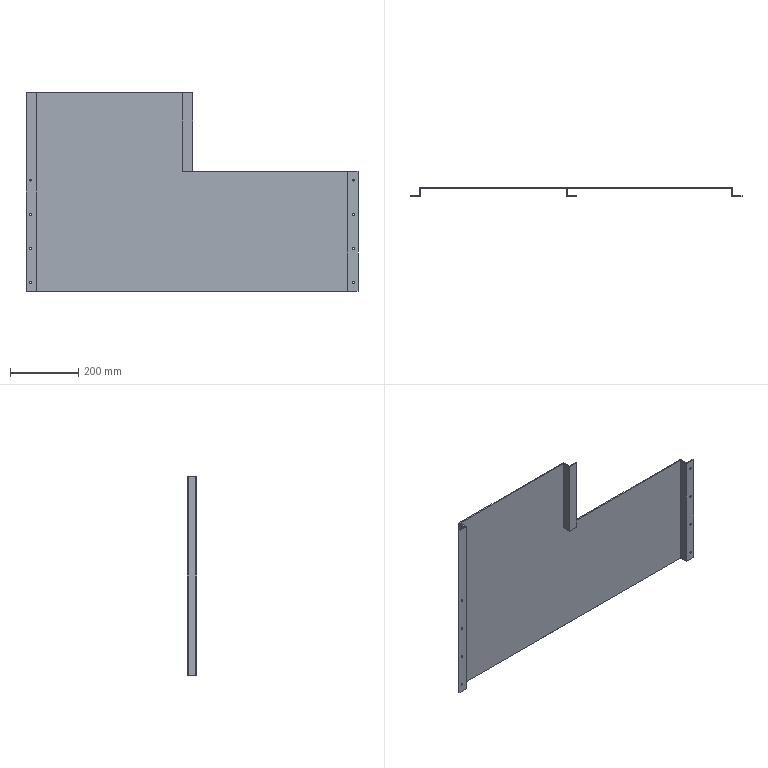Part | STEP file | Cutting guard | 1 solid | 37 faces | box 970 x 28 x 580 mm | volume 1440851 mm3 | plane 21 | cylinder 16 | commonest cylinder face diameters 6 x16
STEP:
#1=CARTESIAN_POINT('',(469.,-25.,-50.));
#2=VERTEX_POINT('',#1);
#3=CARTESIAN_POINT('',(475.,-25.,-50.));
#4=VERTEX_POINT('',#3);
#5=CARTESIAN_POINT('',(472.,-25.,-50.));
#6=DIRECTION('',(0.,-1.,0.));
#7=DIRECTION('',(-1.,0.,0.));
#8=AXIS2_PLACEMENT_3D('',#5,#6,#7);
#9=CIRCLE('',#8,3.);
#10=EDGE_CURVE('',#2,#4,#9,.T.);
#11=ORIENTED_EDGE('',*,*,#10,.T.);
#12=CARTESIAN_POINT('',(475.,-22.,-50.));
#13=VERTEX_POINT('',#12);
#14=CARTESIAN_POINT('',(475.,-372.,-50.));
#15=DIRECTION('',(0.,1.,0.));
#16=VECTOR('',#15,1000.);
#17=LINE('',#14,#16);
#18=EDGE_CURVE('',#4,#13,#17,.T.);
#19=ORIENTED_EDGE('',*,*,#18,.T.);
#20=CARTESIAN_POINT('',(469.,-22.,-50.));
#21=VERTEX_POINT('',#20);
#22=CARTESIAN_POINT('',(472.,-22.,-50.));
#23=DIRECTION('',(0.,-1.,0.));
#24=DIRECTION('',(1.,0.,0.));
#25=AXIS2_PLACEMENT_3D('',#22,#23,#24);
#26=CIRCLE('',#25,3.);
#27=EDGE_CURVE('',#21,#13,#26,.T.);
#28=ORIENTED_EDGE('',*,*,#27,.F.);
#29=CARTESIAN_POINT('',(469.,-372.,-50.));
#30=DIRECTION('',(0.,1.,0.));
#31=VECTOR('',#30,1000.);
#32=LINE('',#29,#31);
#33=EDGE_CURVE('',#2,#21,#32,.T.);
#34=ORIENTED_EDGE('',*,*,#33,.F.);
#35=EDGE_LOOP('',(#11,#19,#28,#34));
#36=FACE_OUTER_BOUND('',#35,.T.);
#37=CARTESIAN_POINT('',(472.,-372.,-50.));
#38=DIRECTION('',(0.,1.,0.));
#39=DIRECTION('',(-1.,0.,0.));
#40=AXIS2_PLACEMENT_3D('',#37,#38,#39);
#41=CYLINDRICAL_SURFACE('',#40,3.);
#42=ADVANCED_FACE('',(#36),#41,.F.);
#43=CARTESIAN_POINT('',(469.,-25.,50.));
#44=VERTEX_POINT('',#43);
#45=CARTESIAN_POINT('',(475.,-25.,50.));
#46=VERTEX_POINT('',#45);
#47=CARTESIAN_POINT('',(472.,-25.,50.));
#48=DIRECTION('',(0.,-1.,0.));
#49=DIRECTION('',(-1.,0.,0.));
#50=AXIS2_PLACEMENT_3D('',#47,#48,#49);
#51=CIRCLE('',#50,3.);
#52=EDGE_CURVE('',#44,#46,#51,.T.);
#53=ORIENTED_EDGE('',*,*,#52,.T.);
#54=CARTESIAN_POINT('',(475.,-22.,50.));
#55=VERTEX_POINT('',#54);
#56=CARTESIAN_POINT('',(475.,-372.,50.));
#57=DIRECTION('',(0.,1.,0.));
#58=VECTOR('',#57,1000.);
#59=LINE('',#56,#58);
#60=EDGE_CURVE('',#46,#55,#59,.T.);
#61=ORIENTED_EDGE('',*,*,#60,.T.);
#62=CARTESIAN_POINT('',(469.,-22.,50.));
#63=VERTEX_POINT('',#62);
#64=CARTESIAN_POINT('',(472.,-22.,50.));
#65=DIRECTION('',(0.,-1.,0.));
#66=DIRECTION('',(1.,0.,0.));
#67=AXIS2_PLACEMENT_3D('',#64,#65,#66);
#68=CIRCLE('',#67,3.);
#69=EDGE_CURVE('',#63,#55,#68,.T.);
#70=ORIENTED_EDGE('',*,*,#69,.F.);
#71=CARTESIAN_POINT('',(469.,-372.,50.));
#72=DIRECTION('',(0.,1.,0.));
#73=VECTOR('',#72,1000.);
#74=LINE('',#71,#73);
#75=EDGE_CURVE('',#44,#63,#74,.T.);
#76=ORIENTED_EDGE('',*,*,#75,.F.);
#77=EDGE_LOOP('',(#53,#61,#70,#76));
#78=FACE_OUTER_BOUND('',#77,.T.);
#79=CARTESIAN_POINT('',(472.,-372.,50.));
#80=DIRECTION('',(0.,1.,0.));
#81=DIRECTION('',(-1.,0.,0.));
#82=AXIS2_PLACEMENT_3D('',#79,#80,#81);
#83=CYLINDRICAL_SURFACE('',#82,3.);
#84=ADVANCED_FACE('',(#78),#83,.F.);
#85=CARTESIAN_POINT('',(469.,-25.,150.));
#86=VERTEX_POINT('',#85);
#87=CARTESIAN_POINT('',(475.,-25.,150.));
#88=VERTEX_POINT('',#87);
#89=CARTESIAN_POINT('',(472.,-25.,150.));
#90=DIRECTION('',(0.,-1.,0.));
#91=DIRECTION('',(-1.,0.,0.));
#92=AXIS2_PLACEMENT_3D('',#89,#90,#91);
#93=CIRCLE('',#92,3.);
#94=EDGE_CURVE('',#86,#88,#93,.T.);
#95=ORIENTED_EDGE('',*,*,#94,.T.);
#96=CARTESIAN_POINT('',(475.,-22.,150.));
#97=VERTEX_POINT('',#96);
#98=CARTESIAN_POINT('',(475.,-372.,150.));
#99=DIRECTION('',(0.,1.,0.));
#100=VECTOR('',#99,1000.);
#101=LINE('',#98,#100);
#102=EDGE_CURVE('',#88,#97,#101,.T.);
#103=ORIENTED_EDGE('',*,*,#102,.T.);
#104=CARTESIAN_POINT('',(469.,-22.,150.));
#105=VERTEX_POINT('',#104);
#106=CARTESIAN_POINT('',(472.,-22.,150.));
#107=DIRECTION('',(0.,-1.,0.));
#108=DIRECTION('',(1.,0.,0.));
#109=AXIS2_PLACEMENT_3D('',#106,#107,#108);
#110=CIRCLE('',#109,3.);
#111=EDGE_CURVE('',#105,#97,#110,.T.);
#112=ORIENTED_EDGE('',*,*,#111,.F.);
#113=CARTESIAN_POINT('',(469.,-372.,150.));
#114=DIRECTION('',(0.,1.,0.));
#115=VECTOR('',#114,1000.);
#116=LINE('',#113,#115);
#117=EDGE_CURVE('',#86,#105,#116,.T.);
#118=ORIENTED_EDGE('',*,*,#117,.F.);
#119=EDGE_LOOP('',(#95,#103,#112,#118));
#120=FACE_OUTER_BOUND('',#119,.T.);
#121=CARTESIAN_POINT('',(472.,-372.,150.));
#122=DIRECTION('',(0.,1.,0.));
#123=DIRECTION('',(-1.,0.,0.));
#124=AXIS2_PLACEMENT_3D('',#121,#122,#123);
#125=CYLINDRICAL_SURFACE('',#124,3.);
#126=ADVANCED_FACE('',(#120),#125,.F.);
#127=CARTESIAN_POINT('',(469.,-25.,-150.));
#128=VERTEX_POINT('',#127);
#129=CARTESIAN_POINT('',(475.,-25.,-150.));
#130=VERTEX_POINT('',#129);
#131=CARTESIAN_POINT('',(472.,-25.,-150.));
#132=DIRECTION('',(0.,-1.,0.));
#133=DIRECTION('',(-1.,0.,0.));
#134=AXIS2_PLACEMENT_3D('',#131,#132,#133);
#135=CIRCLE('',#134,3.);
#136=EDGE_CURVE('',#128,#130,#135,.T.);
#137=ORIENTED_EDGE('',*,*,#136,.T.);
#138=CARTESIAN_POINT('',(475.,-22.,-150.));
#139=VERTEX_POINT('',#138);
#140=CARTESIAN_POINT('',(475.,-372.,-150.));
#141=DIRECTION('',(0.,1.,0.));
#142=VECTOR('',#141,1000.);
#143=LINE('',#140,#142);
#144=EDGE_CURVE('',#130,#139,#143,.T.);
#145=ORIENTED_EDGE('',*,*,#144,.T.);
#146=CARTESIAN_POINT('',(469.,-22.,-150.));
#147=VERTEX_POINT('',#146);
#148=CARTESIAN_POINT('',(472.,-22.,-150.));
#149=DIRECTION('',(0.,-1.,0.));
#150=DIRECTION('',(1.,0.,0.));
#151=AXIS2_PLACEMENT_3D('',#148,#149,#150);
#152=CIRCLE('',#151,3.);
#153=EDGE_CURVE('',#147,#139,#152,.T.);
#154=ORIENTED_EDGE('',*,*,#153,.F.);
#155=CARTESIAN_POINT('',(469.,-372.,-150.));
#156=DIRECTION('',(0.,1.,0.));
#157=VECTOR('',#156,1000.);
#158=LINE('',#155,#157);
#159=EDGE_CURVE('',#128,#147,#158,.T.);
#160=ORIENTED_EDGE('',*,*,#159,.F.);
#161=EDGE_LOOP('',(#137,#145,#154,#160));
#162=FACE_OUTER_BOUND('',#161,.T.);
#163=CARTESIAN_POINT('',(472.,-372.,-150.));
#164=DIRECTION('',(0.,1.,0.));
#165=DIRECTION('',(-1.,0.,0.));
#166=AXIS2_PLACEMENT_3D('',#163,#164,#165);
#167=CYLINDRICAL_SURFACE('',#166,3.);
#168=ADVANCED_FACE('',(#162),#167,.F.);
#169=CARTESIAN_POINT('',(-469.,-25.,150.));
#170=VERTEX_POINT('',#169);
#171=CARTESIAN_POINT('',(-475.,-25.,150.));
#172=VERTEX_POINT('',#171);
#173=CARTESIAN_POINT('',(-472.,-25.,150.));
#174=DIRECTION('',(0.,1.,0.));
#175=DIRECTION('',(-1.,0.,0.));
#176=AXIS2_PLACEMENT_3D('',#173,#174,#175);
#177=CIRCLE('',#176,3.);
#178=EDGE_CURVE('',#170,#172,#177,.T.);
#179=ORIENTED_EDGE('',*,*,#178,.F.);
#180=CARTESIAN_POINT('',(-469.,-22.,150.));
#181=VERTEX_POINT('',#180);
#182=CARTESIAN_POINT('',(-469.,-372.,150.));
#183=DIRECTION('',(0.,1.,0.));
#184=VECTOR('',#183,1000.);
#185=LINE('',#182,#184);
#186=EDGE_CURVE('',#170,#181,#185,.T.);
#187=ORIENTED_EDGE('',*,*,#186,.T.);
#188=CARTESIAN_POINT('',(-475.,-22.,150.));
#189=VERTEX_POINT('',#188);
#190=CARTESIAN_POINT('',(-472.,-22.,150.));
#191=DIRECTION('',(0.,1.,0.));
#192=DIRECTION('',(-1.,0.,0.));
#193=AXIS2_PLACEMENT_3D('',#190,#191,#192);
#194=CIRCLE('',#193,3.);
#195=EDGE_CURVE('',#181,#189,#194,.T.);
#196=ORIENTED_EDGE('',*,*,#195,.T.);
#197=CARTESIAN_POINT('',(-475.,-372.,150.));
#198=DIRECTION('',(0.,1.,0.));
#199=VECTOR('',#198,1000.);
#200=LINE('',#197,#199);
#201=EDGE_CURVE('',#172,#189,#200,.T.);
#202=ORIENTED_EDGE('',*,*,#201,.F.);
#203=EDGE_LOOP('',(#179,#187,#196,#202));
#204=FACE_OUTER_BOUND('',#203,.T.);
#205=CARTESIAN_POINT('',(-472.,-372.,150.));
#206=DIRECTION('',(0.,1.,0.));
#207=DIRECTION('',(-1.,0.,0.));
#208=AXIS2_PLACEMENT_3D('',#205,#206,#207);
#209=CYLINDRICAL_SURFACE('',#208,3.);
#210=ADVANCED_FACE('',(#204),#209,.F.);
#211=CARTESIAN_POINT('',(-469.,-25.,50.));
#212=VERTEX_POINT('',#211);
#213=CARTESIAN_POINT('',(-475.,-25.,50.));
#214=VERTEX_POINT('',#213);
#215=CARTESIAN_POINT('',(-472.,-25.,50.));
#216=DIRECTION('',(0.,1.,0.));
#217=DIRECTION('',(-1.,0.,0.));
#218=AXIS2_PLACEMENT_3D('',#215,#216,#217);
#219=CIRCLE('',#218,3.);
#220=EDGE_CURVE('',#212,#214,#219,.T.);
#221=ORIENTED_EDGE('',*,*,#220,.F.);
#222=CARTESIAN_POINT('',(-469.,-22.,50.));
#223=VERTEX_POINT('',#222);
#224=CARTESIAN_POINT('',(-469.,-372.,50.));
#225=DIRECTION('',(0.,1.,0.));
#226=VECTOR('',#225,1000.);
#227=LINE('',#224,#226);
#228=EDGE_CURVE('',#212,#223,#227,.T.);
#229=ORIENTED_EDGE('',*,*,#228,.T.);
#230=CARTESIAN_POINT('',(-475.,-22.,50.));
#231=VERTEX_POINT('',#230);
#232=CARTESIAN_POINT('',(-472.,-22.,50.));
#233=DIRECTION('',(0.,1.,0.));
#234=DIRECTION('',(-1.,0.,0.));
#235=AXIS2_PLACEMENT_3D('',#232,#233,#234);
#236=CIRCLE('',#235,3.);
#237=EDGE_CURVE('',#223,#231,#236,.T.);
#238=ORIENTED_EDGE('',*,*,#237,.T.);
#239=CARTESIAN_POINT('',(-475.,-372.,50.));
#240=DIRECTION('',(0.,1.,0.));
#241=VECTOR('',#240,1000.);
#242=LINE('',#239,#241);
#243=EDGE_CURVE('',#214,#231,#242,.T.);
#244=ORIENTED_EDGE('',*,*,#243,.F.);
#245=EDGE_LOOP('',(#221,#229,#238,#244));
#246=FACE_OUTER_BOUND('',#245,.T.);
#247=CARTESIAN_POINT('',(-472.,-372.,50.));
#248=DIRECTION('',(0.,1.,0.));
#249=DIRECTION('',(-1.,0.,0.));
#250=AXIS2_PLACEMENT_3D('',#247,#248,#249);
#251=CYLINDRICAL_SURFACE('',#250,3.);
#252=ADVANCED_FACE('',(#246),#251,.F.);
#253=CARTESIAN_POINT('',(-469.,-25.,-50.));
#254=VERTEX_POINT('',#253);
#255=CARTESIAN_POINT('',(-475.,-25.,-50.));
#256=VERTEX_POINT('',#255);
#257=CARTESIAN_POINT('',(-472.,-25.,-50.));
#258=DIRECTION('',(0.,1.,0.));
#259=DIRECTION('',(-1.,0.,0.));
#260=AXIS2_PLACEMENT_3D('',#257,#258,#259);
#261=CIRCLE('',#260,3.);
#262=EDGE_CURVE('',#254,#256,#261,.T.);
#263=ORIENTED_EDGE('',*,*,#262,.F.);
#264=CARTESIAN_POINT('',(-469.,-22.,-50.));
#265=VERTEX_POINT('',#264);
#266=CARTESIAN_POINT('',(-469.,-372.,-50.));
#267=DIRECTION('',(0.,1.,0.));
#268=VECTOR('',#267,1000.);
#269=LINE('',#266,#268);
#270=EDGE_CURVE('',#254,#265,#269,.T.);
#271=ORIENTED_EDGE('',*,*,#270,.T.);
#272=CARTESIAN_POINT('',(-475.,-22.,-50.));
#273=VERTEX_POINT('',#272);
#274=CARTESIAN_POINT('',(-472.,-22.,-50.));
#275=DIRECTION('',(0.,1.,0.));
#276=DIRECTION('',(-1.,0.,0.));
#277=AXIS2_PLACEMENT_3D('',#274,#275,#276);
#278=CIRCLE('',#277,3.);
#279=EDGE_CURVE('',#265,#273,#278,.T.);
#280=ORIENTED_EDGE('',*,*,#279,.T.);
#281=CARTESIAN_POINT('',(-475.,-372.,-50.));
#282=DIRECTION('',(0.,1.,0.));
#283=VECTOR('',#282,1000.);
#284=LINE('',#281,#283);
#285=EDGE_CURVE('',#256,#273,#284,.T.);
#286=ORIENTED_EDGE('',*,*,#285,.F.);
#287=EDGE_LOOP('',(#263,#271,#280,#286));
#288=FACE_OUTER_BOUND('',#287,.T.);
#289=CARTESIAN_POINT('',(-472.,-372.,-50.));
#290=DIRECTION('',(0.,1.,0.));
#291=DIRECTION('',(-1.,0.,0.));
#292=AXIS2_PLACEMENT_3D('',#289,#290,#291);
#293=CYLINDRICAL_SURFACE('',#292,3.);
#294=ADVANCED_FACE('',(#288),#293,.F.);
#295=CARTESIAN_POINT('',(-469.,-25.,-150.));
#296=VERTEX_POINT('',#295);
#297=CARTESIAN_POINT('',(-475.,-25.,-150.));
#298=VERTEX_POINT('',#297);
#299=CARTESIAN_POINT('',(-472.,-25.,-150.));
#300=DIRECTION('',(0.,1.,0.));
#301=DIRECTION('',(-1.,0.,0.));
#302=AXIS2_PLACEMENT_3D('',#299,#300,#301);
#303=CIRCLE('',#302,3.);
#304=EDGE_CURVE('',#296,#298,#303,.T.);
#305=ORIENTED_EDGE('',*,*,#304,.F.);
#306=CARTESIAN_POINT('',(-469.,-22.,-150.));
#307=VERTEX_POINT('',#306);
#308=CARTESIAN_POINT('',(-469.,-372.,-150.));
#309=DIRECTION('',(0.,1.,0.));
#310=VECTOR('',#309,1000.);
#311=LINE('',#308,#310);
#312=EDGE_CURVE('',#296,#307,#311,.T.);
#313=ORIENTED_EDGE('',*,*,#312,.T.);
#314=CARTESIAN_POINT('',(-475.,-22.,-150.));
#315=VERTEX_POINT('',#314);
#316=CARTESIAN_POINT('',(-472.,-22.,-150.));
#317=DIRECTION('',(0.,1.,0.));
#318=DIRECTION('',(-1.,0.,0.));
#319=AXIS2_PLACEMENT_3D('',#316,#317,#318);
#320=CIRCLE('',#319,3.);
#321=EDGE_CURVE('',#307,#315,#320,.T.);
#322=ORIENTED_EDGE('',*,*,#321,.T.);
#323=CARTESIAN_POINT('',(-475.,-372.,-150.));
#324=DIRECTION('',(0.,1.,0.));
#325=VECTOR('',#324,1000.);
#326=LINE('',#323,#325);
#327=EDGE_CURVE('',#298,#315,#326,.T.);
#328=ORIENTED_EDGE('',*,*,#327,.F.);
#329=EDGE_LOOP('',(#305,#313,#322,#328));
#330=FACE_OUTER_BOUND('',#329,.T.);
#331=CARTESIAN_POINT('',(-472.,-372.,-150.));
#332=DIRECTION('',(0.,1.,0.));
#333=DIRECTION('',(-1.,0.,0.));
#334=AXIS2_PLACEMENT_3D('',#331,#332,#333);
#335=CYLINDRICAL_SURFACE('',#334,3.);
#336=ADVANCED_FACE('',(#330),#335,.F.);
#337=CARTESIAN_POINT('',(-25.,0.,175.));
#338=VERTEX_POINT('',#337);
#339=CARTESIAN_POINT('',(-25.,3.,175.));
#340=VERTEX_POINT('',#339);
#341=CARTESIAN_POINT('',(-25.,3.,175.));
#342=DIRECTION('',(0.,1.,0.));
#343=VECTOR('',#342,1000.);
#344=LINE('',#341,#343);
#345=EDGE_CURVE('',#338,#340,#344,.T.);
#346=ORIENTED_EDGE('',*,*,#345,.F.);
#347=CARTESIAN_POINT('',(455.,0.,175.));
#348=VERTEX_POINT('',#347);
#349=CARTESIAN_POINT('',(455.,0.,175.));
#350=DIRECTION('',(1.,0.,0.));
#351=VECTOR('',#350,1000.);
#352=LINE('',#349,#351);
#353=EDGE_CURVE('',#338,#348,#352,.T.);
#354=ORIENTED_EDGE('',*,*,#353,.T.);
#355=CARTESIAN_POINT('',(455.,-25.,175.));
#356=VERTEX_POINT('',#355);
#357=CARTESIAN_POINT('',(455.,0.,175.));
#358=DIRECTION('',(0.,-1.,0.));
#359=VECTOR('',#358,1000.);
#360=LINE('',#357,#359);
#361=EDGE_CURVE('',#348,#356,#360,.T.);
#362=ORIENTED_EDGE('',*,*,#361,.T.);
#363=CARTESIAN_POINT('',(485.,-25.,175.));
#364=VERTEX_POINT('',#363);
#365=CARTESIAN_POINT('',(455.,-25.,175.));
#366=DIRECTION('',(1.,0.,0.));
#367=VECTOR('',#366,1000.);
#368=LINE('',#365,#367);
#369=EDGE_CURVE('',#356,#364,#368,.T.);
#370=ORIENTED_EDGE('',*,*,#369,.T.);
#371=CARTESIAN_POINT('',(485.,-22.,175.));
#372=VERTEX_POINT('',#371);
#373=CARTESIAN_POINT('',(485.,-25.,175.));
#374=DIRECTION('',(0.,1.,0.));
#375=VECTOR('',#374,1000.);
#376=LINE('',#373,#375);
#377=EDGE_CURVE('',#364,#372,#376,.T.);
#378=ORIENTED_EDGE('',*,*,#377,.T.);
#379=CARTESIAN_POINT('',(458.,-22.,175.));
#380=VERTEX_POINT('',#379);
#381=CARTESIAN_POINT('',(458.,-22.,175.));
#382=DIRECTION('',(-1.,0.,0.));
#383=VECTOR('',#382,1000.);
#384=LINE('',#381,#383);
#385=EDGE_CURVE('',#372,#380,#384,.T.);
#386=ORIENTED_EDGE('',*,*,#385,.T.);
#387=CARTESIAN_POINT('',(458.,3.,175.));
#388=VERTEX_POINT('',#387);
#389=CARTESIAN_POINT('',(458.,3.,175.));
#390=DIRECTION('',(0.,1.,0.));
#391=VECTOR('',#390,1000.);
#392=LINE('',#389,#391);
#393=EDGE_CURVE('',#380,#388,#392,.T.);
#394=ORIENTED_EDGE('',*,*,#393,.T.);
#395=CARTESIAN_POINT('',(458.,3.,175.));
#396=DIRECTION('',(-1.,0.,0.));
#397=VECTOR('',#396,1000.);
#398=LINE('',#395,#397);
#399=EDGE_CURVE('',#388,#340,#398,.T.);
#400=ORIENTED_EDGE('',*,*,#399,.T.);
#401=EDGE_LOOP('',(#346,#354,#362,#370,#378,#386,#394,#400));
#402=FACE_OUTER_BOUND('',#401,.T.);
#403=CARTESIAN_POINT('',(0.,0.,175.));
#404=DIRECTION('',(0.,0.,-1.));
#405=DIRECTION('',(-1.,0.,0.));
#406=AXIS2_PLACEMENT_3D('',#403,#404,#405);
#407=PLANE('',#406);
#408=ADVANCED_FACE('',(#402),#407,.F.);
#409=CARTESIAN_POINT('',(-455.,-25.,-175.));
#410=VERTEX_POINT('',#409);
#411=CARTESIAN_POINT('',(-455.,0.,-175.));
#412=VERTEX_POINT('',#411);
#413=CARTESIAN_POINT('',(-455.,0.,-175.));
#414=DIRECTION('',(0.,1.,0.));
#415=VECTOR('',#414,1000.);
#416=LINE('',#413,#415);
#417=EDGE_CURVE('',#410,#412,#416,.T.);
#418=ORIENTED_EDGE('',*,*,#417,.T.);
#419=CARTESIAN_POINT('',(-455.,0.,405.));
#420=VERTEX_POINT('',#419);
#421=CARTESIAN_POINT('',(-455.,0.,175.));
#422=DIRECTION('',(0.,0.,-1.));
#423=VECTOR('',#422,1000.);
#424=LINE('',#421,#423);
#425=EDGE_CURVE('',#420,#412,#424,.T.);
#426=ORIENTED_EDGE('',*,*,#425,.F.);
#427=CARTESIAN_POINT('',(-455.,-25.,405.));
#428=VERTEX_POINT('',#427);
#429=CARTESIAN_POINT('',(-455.,-25.,405.));
#430=DIRECTION('',(0.,1.,0.));
#431=VECTOR('',#430,1000.);
#432=LINE('',#429,#431);
#433=EDGE_CURVE('',#428,#420,#432,.T.);
#434=ORIENTED_EDGE('',*,*,#433,.F.);
#435=CARTESIAN_POINT('',(-455.,-25.,175.));
#436=DIRECTION('',(0.,0.,-1.));
#437=VECTOR('',#436,1000.);
#438=LINE('',#435,#437);
#439=EDGE_CURVE('',#428,#410,#438,.T.);
#440=ORIENTED_EDGE('',*,*,#439,.T.);
#441=EDGE_LOOP('',(#418,#426,#434,#440));
#442=FACE_OUTER_BOUND('',#441,.T.);
#443=CARTESIAN_POINT('',(-455.,0.,175.));
#444=DIRECTION('',(-1.,0.,0.));
#445=DIRECTION('',(0.,0.,1.));
#446=AXIS2_PLACEMENT_3D('',#443,#444,#445);
#447=PLANE('',#446);
#448=ADVANCED_FACE('',(#442),#447,.F.);
#449=CARTESIAN_POINT('',(455.,0.,-175.));
#450=VERTEX_POINT('',#449);
#451=CARTESIAN_POINT('',(455.,0.,-175.));
#452=DIRECTION('',(1.,0.,0.));
#453=VECTOR('',#452,1000.);
#454=LINE('',#451,#453);
#455=EDGE_CURVE('',#412,#450,#454,.T.);
#456=ORIENTED_EDGE('',*,*,#455,.T.);
#457=CARTESIAN_POINT('',(455.,0.,175.));
#458=DIRECTION('',(0.,0.,-1.));
#459=VECTOR('',#458,1000.);
#460=LINE('',#457,#459);
#461=EDGE_CURVE('',#348,#450,#460,.T.);
#462=ORIENTED_EDGE('',*,*,#461,.F.);
#463=ORIENTED_EDGE('',*,*,#353,.F.);
#464=CARTESIAN_POINT('',(-28.,0.,175.));
#465=VERTEX_POINT('',#464);
#466=CARTESIAN_POINT('',(455.,0.,175.));
#467=DIRECTION('',(1.,0.,0.));
#468=VECTOR('',#467,1000.);
#469=LINE('',#466,#468);
#470=EDGE_CURVE('',#465,#338,#469,.T.);
#471=ORIENTED_EDGE('',*,*,#470,.F.);
#472=CARTESIAN_POINT('',(-28.,0.,405.));
#473=VERTEX_POINT('',#472);
#474=CARTESIAN_POINT('',(-28.,0.,405.));
#475=DIRECTION('',(0.,0.,-1.));
#476=VECTOR('',#475,1000.);
#477=LINE('',#474,#476);
#478=EDGE_CURVE('',#473,#465,#477,.T.);
#479=ORIENTED_EDGE('',*,*,#478,.F.);
#480=CARTESIAN_POINT('',(-28.,0.,405.));
#481=DIRECTION('',(1.,0.,0.));
#482=VECTOR('',#481,1000.);
#483=LINE('',#480,#482);
#484=EDGE_CURVE('',#420,#473,#483,.T.);
#485=ORIENTED_EDGE('',*,*,#484,.F.);
#486=ORIENTED_EDGE('',*,*,#425,.T.);
#487=EDGE_LOOP('',(#456,#462,#463,#471,#479,#485,#486));
#488=FACE_OUTER_BOUND('',#487,.T.);
#489=CARTESIAN_POINT('',(455.,0.,175.));
#490=DIRECTION('',(0.,1.,0.));
#491=DIRECTION('',(0.,0.,1.));
#492=AXIS2_PLACEMENT_3D('',#489,#490,#491);
#493=PLANE('',#492);
#494=ADVANCED_FACE('',(#488),#493,.F.);
#495=CARTESIAN_POINT('',(455.,-25.,-175.));
#496=VERTEX_POINT('',#495);
#497=CARTESIAN_POINT('',(455.,0.,-175.));
#498=DIRECTION('',(0.,-1.,0.));
#499=VECTOR('',#498,1000.);
#500=LINE('',#497,#499);
#501=EDGE_CURVE('',#450,#496,#500,.T.);
#502=ORIENTED_EDGE('',*,*,#501,.T.);
#503=CARTESIAN_POINT('',(455.,-25.,175.));
#504=DIRECTION('',(0.,0.,-1.));
#505=VECTOR('',#504,1000.);
#506=LINE('',#503,#505);
#507=EDGE_CURVE('',#356,#496,#506,.T.);
#508=ORIENTED_EDGE('',*,*,#507,.F.);
#509=ORIENTED_EDGE('',*,*,#361,.F.);
#510=ORIENTED_EDGE('',*,*,#461,.T.);
#511=EDGE_LOOP('',(#502,#508,#509,#510));
#512=FACE_OUTER_BOUND('',#511,.T.);
#513=CARTESIAN_POINT('',(455.,0.,175.));
#514=DIRECTION('',(1.,0.,0.));
#515=DIRECTION('',(0.,0.,-1.));
#516=AXIS2_PLACEMENT_3D('',#513,#514,#515);
#517=PLANE('',#516);
#518=ADVANCED_FACE('',(#512),#517,.F.);
#519=ORIENTED_EDGE('',*,*,#10,.F.);
#520=CARTESIAN_POINT('',(472.,-25.,-50.));
#521=DIRECTION('',(0.,-1.,0.));
#522=DIRECTION('',(-1.,0.,0.));
#523=AXIS2_PLACEMENT_3D('',#520,#521,#522);
#524=CIRCLE('',#523,3.);
#525=EDGE_CURVE('',#4,#2,#524,.T.);
#526=ORIENTED_EDGE('',*,*,#525,.F.);
#527=EDGE_LOOP('',(#519,#526));
#528=FACE_BOUND('',#527,.T.);
#529=ORIENTED_EDGE('',*,*,#52,.F.);
#530=CARTESIAN_POINT('',(472.,-25.,50.));
#531=DIRECTION('',(0.,-1.,0.));
#532=DIRECTION('',(-1.,0.,0.));
#533=AXIS2_PLACEMENT_3D('',#530,#531,#532);
#534=CIRCLE('',#533,3.);
#535=EDGE_CURVE('',#46,#44,#534,.T.);
#536=ORIENTED_EDGE('',*,*,#535,.F.);
#537=EDGE_LOOP('',(#529,#536));
#538=FACE_BOUND('',#537,.T.);
#539=ORIENTED_EDGE('',*,*,#94,.F.);
#540=CARTESIAN_POINT('',(472.,-25.,150.));
#541=DIRECTION('',(0.,-1.,0.));
#542=DIRECTION('',(-1.,0.,0.));
#543=AXIS2_PLACEMENT_3D('',#540,#541,#542);
#544=CIRCLE('',#543,3.);
#545=EDGE_CURVE('',#88,#86,#544,.T.);
#546=ORIENTED_EDGE('',*,*,#545,.F.);
#547=EDGE_LOOP('',(#539,#546));
#548=FACE_BOUND('',#547,.T.);
#549=ORIENTED_EDGE('',*,*,#136,.F.);
#550=CARTESIAN_POINT('',(472.,-25.,-150.));
#551=DIRECTION('',(0.,-1.,0.));
#552=DIRECTION('',(-1.,0.,0.));
#553=AXIS2_PLACEMENT_3D('',#550,#551,#552);
#554=CIRCLE('',#553,3.);
#555=EDGE_CURVE('',#130,#128,#554,.T.);
#556=ORIENTED_EDGE('',*,*,#555,.F.);
#557=EDGE_LOOP('',(#549,#556));
#558=FACE_BOUND('',#557,.T.);
#559=CARTESIAN_POINT('',(485.,-25.,-175.));
#560=VERTEX_POINT('',#559);
#561=CARTESIAN_POINT('',(455.,-25.,-175.));
#562=DIRECTION('',(1.,0.,0.));
#563=VECTOR('',#562,1000.);
#564=LINE('',#561,#563);
#565=EDGE_CURVE('',#496,#560,#564,.T.);
#566=ORIENTED_EDGE('',*,*,#565,.T.);
#567=CARTESIAN_POINT('',(485.,-25.,175.));
#568=DIRECTION('',(0.,0.,-1.));
#569=VECTOR('',#568,1000.);
#570=LINE('',#567,#569);
#571=EDGE_CURVE('',#364,#560,#570,.T.);
#572=ORIENTED_EDGE('',*,*,#571,.F.);
#573=ORIENTED_EDGE('',*,*,#369,.F.);
#574=ORIENTED_EDGE('',*,*,#507,.T.);
#575=EDGE_LOOP('',(#566,#572,#573,#574));
#576=FACE_OUTER_BOUND('',#575,.T.);
#577=CARTESIAN_POINT('',(455.,-25.,175.));
#578=DIRECTION('',(0.,1.,0.));
#579=DIRECTION('',(-1.,0.,0.));
#580=AXIS2_PLACEMENT_3D('',#577,#578,#579);
#581=PLANE('',#580);
#582=ADVANCED_FACE('',(#528,#538,#548,#558,#576),#581,.F.);
#583=CARTESIAN_POINT('',(485.,-22.,-175.));
#584=VERTEX_POINT('',#583);
#585=CARTESIAN_POINT('',(485.,-25.,-175.));
#586=DIRECTION('',(0.,1.,0.));
#587=VECTOR('',#586,1000.);
#588=LINE('',#585,#587);
#589=EDGE_CURVE('',#560,#584,#588,.T.);
#590=ORIENTED_EDGE('',*,*,#589,.T.);
#591=CARTESIAN_POINT('',(485.,-22.,175.));
#592=DIRECTION('',(0.,0.,-1.));
#593=VECTOR('',#592,1000.);
#594=LINE('',#591,#593);
#595=EDGE_CURVE('',#372,#584,#594,.T.);
#596=ORIENTED_EDGE('',*,*,#595,.F.);
#597=ORIENTED_EDGE('',*,*,#377,.F.);
#598=ORIENTED_EDGE('',*,*,#571,.T.);
#599=EDGE_LOOP('',(#590,#596,#597,#598));
#600=FACE_OUTER_BOUND('',#599,.T.);
#601=CARTESIAN_POINT('',(485.,-25.,175.));
#602=DIRECTION('',(-1.,0.,0.));
#603=DIRECTION('',(0.,0.,1.));
#604=AXIS2_PLACEMENT_3D('',#601,#602,#603);
#605=PLANE('',#604);
#606=ADVANCED_FACE('',(#600),#605,.F.);
#607=ORIENTED_EDGE('',*,*,#27,.T.);
#608=CARTESIAN_POINT('',(472.,-22.,-50.));
#609=DIRECTION('',(0.,-1.,0.));
#610=DIRECTION('',(1.,0.,0.));
#611=AXIS2_PLACEMENT_3D('',#608,#609,#610);
#612=CIRCLE('',#611,3.);
#613=EDGE_CURVE('',#13,#21,#612,.T.);
#614=ORIENTED_EDGE('',*,*,#613,.T.);
#615=EDGE_LOOP('',(#607,#614));
#616=FACE_BOUND('',#615,.T.);
#617=ORIENTED_EDGE('',*,*,#69,.T.);
#618=CARTESIAN_POINT('',(472.,-22.,50.));
#619=DIRECTION('',(0.,-1.,0.));
#620=DIRECTION('',(1.,0.,0.));
#621=AXIS2_PLACEMENT_3D('',#618,#619,#620);
#622=CIRCLE('',#621,3.);
#623=EDGE_CURVE('',#55,#63,#622,.T.);
#624=ORIENTED_EDGE('',*,*,#623,.T.);
#625=EDGE_LOOP('',(#617,#624));
#626=FACE_BOUND('',#625,.T.);
#627=ORIENTED_EDGE('',*,*,#111,.T.);
#628=CARTESIAN_POINT('',(472.,-22.,150.));
#629=DIRECTION('',(0.,-1.,0.));
#630=DIRECTION('',(1.,0.,0.));
#631=AXIS2_PLACEMENT_3D('',#628,#629,#630);
#632=CIRCLE('',#631,3.);
#633=EDGE_CURVE('',#97,#105,#632,.T.);
#634=ORIENTED_EDGE('',*,*,#633,.T.);
#635=EDGE_LOOP('',(#627,#634));
#636=FACE_BOUND('',#635,.T.);
#637=ORIENTED_EDGE('',*,*,#153,.T.);
#638=CARTESIAN_POINT('',(472.,-22.,-150.));
#639=DIRECTION('',(0.,-1.,0.));
#640=DIRECTION('',(1.,0.,0.));
#641=AXIS2_PLACEMENT_3D('',#638,#639,#640);
#642=CIRCLE('',#641,3.);
#643=EDGE_CURVE('',#139,#147,#642,.T.);
#644=ORIENTED_EDGE('',*,*,#643,.T.);
#645=EDGE_LOOP('',(#637,#644));
#646=FACE_BOUND('',#645,.T.);
#647=CARTESIAN_POINT('',(458.,-22.,-175.));
#648=VERTEX_POINT('',#647);
#649=CARTESIAN_POINT('',(458.,-22.,-175.));
#650=DIRECTION('',(-1.,0.,0.));
#651=VECTOR('',#650,1000.);
#652=LINE('',#649,#651);
#653=EDGE_CURVE('',#584,#648,#652,.T.);
#654=ORIENTED_EDGE('',*,*,#653,.T.);
#655=CARTESIAN_POINT('',(458.,-22.,175.));
#656=DIRECTION('',(0.,0.,-1.));
#657=VECTOR('',#656,1000.);
#658=LINE('',#655,#657);
#659=EDGE_CURVE('',#380,#648,#658,.T.);
#660=ORIENTED_EDGE('',*,*,#659,.F.);
#661=ORIENTED_EDGE('',*,*,#385,.F.);
#662=ORIENTED_EDGE('',*,*,#595,.T.);
#663=EDGE_LOOP('',(#654,#660,#661,#662));
#664=FACE_OUTER_BOUND('',#663,.T.);
#665=CARTESIAN_POINT('',(458.,-22.,175.));
#666=DIRECTION('',(0.,-1.,0.));
#667=DIRECTION('',(1.,0.,0.));
#668=AXIS2_PLACEMENT_3D('',#665,#666,#667);
#669=PLANE('',#668);
#670=ADVANCED_FACE('',(#616,#626,#636,#646,#664),#669,.F.);
#671=CARTESIAN_POINT('',(458.,3.,-175.));
#672=VERTEX_POINT('',#671);
#673=CARTESIAN_POINT('',(458.,3.,-175.));
#674=DIRECTION('',(0.,1.,0.));
#675=VECTOR('',#674,1000.);
#676=LINE('',#673,#675);
#677=EDGE_CURVE('',#648,#672,#676,.T.);
#678=ORIENTED_EDGE('',*,*,#677,.T.);
#679=CARTESIAN_POINT('',(458.,3.,175.));
#680=DIRECTION('',(0.,0.,-1.));
#681=VECTOR('',#680,1000.);
#682=LINE('',#679,#681);
#683=EDGE_CURVE('',#388,#672,#682,.T.);
#684=ORIENTED_EDGE('',*,*,#683,.F.);
#685=ORIENTED_EDGE('',*,*,#393,.F.);
#686=ORIENTED_EDGE('',*,*,#659,.T.);
#687=EDGE_LOOP('',(#678,#684,#685,#686));
#688=FACE_OUTER_BOUND('',#687,.T.);
#689=CARTESIAN_POINT('',(458.,3.,175.));
#690=DIRECTION('',(-1.,0.,0.));
#691=DIRECTION('',(0.,0.,1.));
#692=AXIS2_PLACEMENT_3D('',#689,#690,#691);
#693=PLANE('',#692);
#694=ADVANCED_FACE('',(#688),#693,.F.);
#695=CARTESIAN_POINT('',(-458.,3.,-175.));
#696=VERTEX_POINT('',#695);
#697=CARTESIAN_POINT('',(458.,3.,-175.));
#698=DIRECTION('',(-1.,0.,0.));
#699=VECTOR('',#698,1000.);
#700=LINE('',#697,#699);
#701=EDGE_CURVE('',#672,#696,#700,.T.);
#702=ORIENTED_EDGE('',*,*,#701,.T.);
#703=CARTESIAN_POINT('',(-458.,3.,405.));
#704=VERTEX_POINT('',#703);
#705=CARTESIAN_POINT('',(-458.,3.,175.));
#706=DIRECTION('',(0.,0.,-1.));
#707=VECTOR('',#706,1000.);
#708=LINE('',#705,#707);
#709=EDGE_CURVE('',#704,#696,#708,.T.);
#710=ORIENTED_EDGE('',*,*,#709,.F.);
#711=CARTESIAN_POINT('',(-25.,3.,405.));
#712=VERTEX_POINT('',#711);
#713=CARTESIAN_POINT('',(-25.,3.,405.));
#714=DIRECTION('',(-1.,0.,0.));
#715=VECTOR('',#714,1000.);
#716=LINE('',#713,#715);
#717=EDGE_CURVE('',#712,#704,#716,.T.);
#718=ORIENTED_EDGE('',*,*,#717,.F.);
#719=CARTESIAN_POINT('',(-25.,3.,405.));
#720=DIRECTION('',(0.,0.,-1.));
#721=VECTOR('',#720,1000.);
#722=LINE('',#719,#721);
#723=EDGE_CURVE('',#712,#340,#722,.T.);
#724=ORIENTED_EDGE('',*,*,#723,.T.);
#725=ORIENTED_EDGE('',*,*,#399,.F.);
#726=ORIENTED_EDGE('',*,*,#683,.T.);
#727=EDGE_LOOP('',(#702,#710,#718,#724,#725,#726));
#728=FACE_OUTER_BOUND('',#727,.T.);
#729=CARTESIAN_POINT('',(458.,3.,175.));
#730=DIRECTION('',(0.,-1.,0.));
#731=DIRECTION('',(1.,0.,0.));
#732=AXIS2_PLACEMENT_3D('',#729,#730,#731);
#733=PLANE('',#732);
#734=ADVANCED_FACE('',(#728),#733,.F.);
#735=CARTESIAN_POINT('',(-458.,-22.,-175.));
#736=VERTEX_POINT('',#735);
#737=CARTESIAN_POINT('',(-458.,3.,-175.));
#738=DIRECTION('',(0.,-1.,0.));
#739=VECTOR('',#738,1000.);
#740=LINE('',#737,#739);
#741=EDGE_CURVE('',#696,#736,#740,.T.);
#742=ORIENTED_EDGE('',*,*,#741,.T.);
#743=CARTESIAN_POINT('',(-458.,-22.,405.));
#744=VERTEX_POINT('',#743);
#745=CARTESIAN_POINT('',(-458.,-22.,175.));
#746=DIRECTION('',(0.,0.,-1.));
#747=VECTOR('',#746,1000.);
#748=LINE('',#745,#747);
#749=EDGE_CURVE('',#744,#736,#748,.T.);
#750=ORIENTED_EDGE('',*,*,#749,.F.);
#751=CARTESIAN_POINT('',(-458.,3.,405.));
#752=DIRECTION('',(0.,-1.,0.));
#753=VECTOR('',#752,1000.);
#754=LINE('',#751,#753);
#755=EDGE_CURVE('',#704,#744,#754,.T.);
#756=ORIENTED_EDGE('',*,*,#755,.F.);
#757=ORIENTED_EDGE('',*,*,#709,.T.);
#758=EDGE_LOOP('',(#742,#750,#756,#757));
#759=FACE_OUTER_BOUND('',#758,.T.);
#760=CARTESIAN_POINT('',(-458.,3.,175.));
#761=DIRECTION('',(1.,0.,0.));
#762=DIRECTION('',(0.,0.,-1.));
#763=AXIS2_PLACEMENT_3D('',#760,#761,#762);
#764=PLANE('',#763);
#765=ADVANCED_FACE('',(#759),#764,.F.);
#766=CARTESIAN_POINT('',(-472.,-22.,-50.));
#767=DIRECTION('',(0.,1.,0.));
#768=DIRECTION('',(-1.,0.,0.));
#769=AXIS2_PLACEMENT_3D('',#766,#767,#768);
#770=CIRCLE('',#769,3.);
#771=EDGE_CURVE('',#273,#265,#770,.T.);
#772=ORIENTED_EDGE('',*,*,#771,.F.);
#773=ORIENTED_EDGE('',*,*,#279,.F.);
#774=EDGE_LOOP('',(#772,#773));
#775=FACE_BOUND('',#774,.T.);
#776=CARTESIAN_POINT('',(-472.,-22.,-150.));
#777=DIRECTION('',(0.,1.,0.));
#778=DIRECTION('',(-1.,0.,0.));
#779=AXIS2_PLACEMENT_3D('',#776,#777,#778);
#780=CIRCLE('',#779,3.);
#781=EDGE_CURVE('',#315,#307,#780,.T.);
#782=ORIENTED_EDGE('',*,*,#781,.F.);
#783=ORIENTED_EDGE('',*,*,#321,.F.);
#784=EDGE_LOOP('',(#782,#783));
#785=FACE_BOUND('',#784,.T.);
#786=CARTESIAN_POINT('',(-485.,-22.,-175.));
#787=VERTEX_POINT('',#786);
#788=CARTESIAN_POINT('',(-458.,-22.,-175.));
#789=DIRECTION('',(-1.,0.,0.));
#790=VECTOR('',#789,1000.);
#791=LINE('',#788,#790);
#792=EDGE_CURVE('',#736,#787,#791,.T.);
#793=ORIENTED_EDGE('',*,*,#792,.T.);
#794=CARTESIAN_POINT('',(-485.,-22.,405.));
#795=VERTEX_POINT('',#794);
#796=CARTESIAN_POINT('',(-485.,-22.,175.));
#797=DIRECTION('',(0.,0.,-1.));
#798=VECTOR('',#797,1000.);
#799=LINE('',#796,#798);
#800=EDGE_CURVE('',#795,#787,#799,.T.);
#801=ORIENTED_EDGE('',*,*,#800,.F.);
#802=CARTESIAN_POINT('',(-458.,-22.,405.));
#803=DIRECTION('',(-1.,0.,0.));
#804=VECTOR('',#803,1000.);
#805=LINE('',#802,#804);
#806=EDGE_CURVE('',#744,#795,#805,.T.);
#807=ORIENTED_EDGE('',*,*,#806,.F.);
#808=ORIENTED_EDGE('',*,*,#749,.T.);
#809=EDGE_LOOP('',(#793,#801,#807,#808));
#810=FACE_OUTER_BOUND('',#809,.T.);
#811=CARTESIAN_POINT('',(-472.,-22.,50.));
#812=DIRECTION('',(0.,1.,0.));
#813=DIRECTION('',(-1.,0.,0.));
#814=AXIS2_PLACEMENT_3D('',#811,#812,#813);
#815=CIRCLE('',#814,3.);
#816=EDGE_CURVE('',#231,#223,#815,.T.);
#817=ORIENTED_EDGE('',*,*,#816,.F.);
#818=ORIENTED_EDGE('',*,*,#237,.F.);
#819=EDGE_LOOP('',(#817,#818));
#820=FACE_BOUND('',#819,.T.);
#821=CARTESIAN_POINT('',(-472.,-22.,150.));
#822=DIRECTION('',(0.,1.,0.));
#823=DIRECTION('',(-1.,0.,0.));
#824=AXIS2_PLACEMENT_3D('',#821,#822,#823);
#825=CIRCLE('',#824,3.);
#826=EDGE_CURVE('',#189,#181,#825,.T.);
#827=ORIENTED_EDGE('',*,*,#826,.F.);
#828=ORIENTED_EDGE('',*,*,#195,.F.);
#829=EDGE_LOOP('',(#827,#828));
#830=FACE_BOUND('',#829,.T.);
#831=CARTESIAN_POINT('',(-458.,-22.,175.));
#832=DIRECTION('',(0.,-1.,0.));
#833=DIRECTION('',(1.,0.,0.));
#834=AXIS2_PLACEMENT_3D('',#831,#832,#833);
#835=PLANE('',#834);
#836=ADVANCED_FACE('',(#775,#785,#810,#820,#830),#835,.F.);
#837=CARTESIAN_POINT('',(-485.,-25.,-175.));
#838=VERTEX_POINT('',#837);
#839=CARTESIAN_POINT('',(-485.,-25.,-175.));
#840=DIRECTION('',(0.,-1.,0.));
#841=VECTOR('',#840,1000.);
#842=LINE('',#839,#841);
#843=EDGE_CURVE('',#787,#838,#842,.T.);
#844=ORIENTED_EDGE('',*,*,#843,.T.);
#845=CARTESIAN_POINT('',(-485.,-25.,405.));
#846=VERTEX_POINT('',#845);
#847=CARTESIAN_POINT('',(-485.,-25.,175.));
#848=DIRECTION('',(0.,0.,-1.));
#849=VECTOR('',#848,1000.);
#850=LINE('',#847,#849);
#851=EDGE_CURVE('',#846,#838,#850,.T.);
#852=ORIENTED_EDGE('',*,*,#851,.F.);
#853=CARTESIAN_POINT('',(-485.,-22.,405.));
#854=DIRECTION('',(0.,-1.,0.));
#855=VECTOR('',#854,1000.);
#856=LINE('',#853,#855);
#857=EDGE_CURVE('',#795,#846,#856,.T.);
#858=ORIENTED_EDGE('',*,*,#857,.F.);
#859=ORIENTED_EDGE('',*,*,#800,.T.);
#860=EDGE_LOOP('',(#844,#852,#858,#859));
#861=FACE_OUTER_BOUND('',#860,.T.);
#862=CARTESIAN_POINT('',(-485.,-25.,175.));
#863=DIRECTION('',(1.,0.,0.));
#864=DIRECTION('',(0.,0.,-1.));
#865=AXIS2_PLACEMENT_3D('',#862,#863,#864);
#866=PLANE('',#865);
#867=ADVANCED_FACE('',(#861),#866,.F.);
#868=CARTESIAN_POINT('',(-472.,-25.,-50.));
#869=DIRECTION('',(0.,1.,0.));
#870=DIRECTION('',(-1.,0.,0.));
#871=AXIS2_PLACEMENT_3D('',#868,#869,#870);
#872=CIRCLE('',#871,3.);
#873=EDGE_CURVE('',#256,#254,#872,.T.);
#874=ORIENTED_EDGE('',*,*,#873,.T.);
#875=ORIENTED_EDGE('',*,*,#262,.T.);
#876=EDGE_LOOP('',(#874,#875));
#877=FACE_BOUND('',#876,.T.);
#878=CARTESIAN_POINT('',(-472.,-25.,-150.));
#879=DIRECTION('',(0.,1.,0.));
#880=DIRECTION('',(-1.,0.,0.));
#881=AXIS2_PLACEMENT_3D('',#878,#879,#880);
#882=CIRCLE('',#881,3.);
#883=EDGE_CURVE('',#298,#296,#882,.T.);
#884=ORIENTED_EDGE('',*,*,#883,.T.);
#885=ORIENTED_EDGE('',*,*,#304,.T.);
#886=EDGE_LOOP('',(#884,#885));
#887=FACE_BOUND('',#886,.T.);
#888=CARTESIAN_POINT('',(-455.,-25.,-175.));
#889=DIRECTION('',(1.,0.,0.));
#890=VECTOR('',#889,1000.);
#891=LINE('',#888,#890);
#892=EDGE_CURVE('',#838,#410,#891,.T.);
#893=ORIENTED_EDGE('',*,*,#892,.T.);
#894=ORIENTED_EDGE('',*,*,#439,.F.);
#895=CARTESIAN_POINT('',(-485.,-25.,405.));
#896=DIRECTION('',(1.,0.,0.));
#897=VECTOR('',#896,1000.);
#898=LINE('',#895,#897);
#899=EDGE_CURVE('',#846,#428,#898,.T.);
#900=ORIENTED_EDGE('',*,*,#899,.F.);
#901=ORIENTED_EDGE('',*,*,#851,.T.);
#902=EDGE_LOOP('',(#893,#894,#900,#901));
#903=FACE_OUTER_BOUND('',#902,.T.);
#904=CARTESIAN_POINT('',(-472.,-25.,50.));
#905=DIRECTION('',(0.,1.,0.));
#906=DIRECTION('',(-1.,0.,0.));
#907=AXIS2_PLACEMENT_3D('',#904,#905,#906);
#908=CIRCLE('',#907,3.);
#909=EDGE_CURVE('',#214,#212,#908,.T.);
#910=ORIENTED_EDGE('',*,*,#909,.T.);
#911=ORIENTED_EDGE('',*,*,#220,.T.);
#912=EDGE_LOOP('',(#910,#911));
#913=FACE_BOUND('',#912,.T.);
#914=CARTESIAN_POINT('',(-472.,-25.,150.));
#915=DIRECTION('',(0.,1.,0.));
#916=DIRECTION('',(-1.,0.,0.));
#917=AXIS2_PLACEMENT_3D('',#914,#915,#916);
#918=CIRCLE('',#917,3.);
#919=EDGE_CURVE('',#172,#170,#918,.T.);
#920=ORIENTED_EDGE('',*,*,#919,.T.);
#921=ORIENTED_EDGE('',*,*,#178,.T.);
#922=EDGE_LOOP('',(#920,#921));
#923=FACE_BOUND('',#922,.T.);
#924=CARTESIAN_POINT('',(-455.,-25.,175.));
#925=DIRECTION('',(0.,1.,0.));
#926=DIRECTION('',(-1.,0.,0.));
#927=AXIS2_PLACEMENT_3D('',#924,#925,#926);
#928=PLANE('',#927);
#929=ADVANCED_FACE('',(#877,#887,#903,#913,#923),#928,.F.);
#930=ORIENTED_EDGE('',*,*,#417,.F.);
#931=ORIENTED_EDGE('',*,*,#892,.F.);
#932=ORIENTED_EDGE('',*,*,#843,.F.);
#933=ORIENTED_EDGE('',*,*,#792,.F.);
#934=ORIENTED_EDGE('',*,*,#741,.F.);
#935=ORIENTED_EDGE('',*,*,#701,.F.);
#936=ORIENTED_EDGE('',*,*,#677,.F.);
#937=ORIENTED_EDGE('',*,*,#653,.F.);
#938=ORIENTED_EDGE('',*,*,#589,.F.);
#939=ORIENTED_EDGE('',*,*,#565,.F.);
#940=ORIENTED_EDGE('',*,*,#501,.F.);
#941=ORIENTED_EDGE('',*,*,#455,.F.);
#942=EDGE_LOOP('',(#930,#931,#932,#933,#934,#935,#936,#937,#938,#939,#940,#941));
#943=FACE_OUTER_BOUND('',#942,.T.);
#944=CARTESIAN_POINT('',(0.,0.,-175.));
#945=DIRECTION('',(0.,0.,-1.));
#946=DIRECTION('',(-1.,0.,0.));
#947=AXIS2_PLACEMENT_3D('',#944,#945,#946);
#948=PLANE('',#947);
#949=ADVANCED_FACE('',(#943),#948,.T.);
#950=ORIENTED_EDGE('',*,*,#312,.F.);
#951=ORIENTED_EDGE('',*,*,#883,.F.);
#952=ORIENTED_EDGE('',*,*,#327,.T.);
#953=ORIENTED_EDGE('',*,*,#781,.T.);
#954=EDGE_LOOP('',(#950,#951,#952,#953));
#955=FACE_OUTER_BOUND('',#954,.T.);
#956=CARTESIAN_POINT('',(-472.,-372.,-150.));
#957=DIRECTION('',(0.,1.,0.));
#958=DIRECTION('',(-1.,0.,0.));
#959=AXIS2_PLACEMENT_3D('',#956,#957,#958);
#960=CYLINDRICAL_SURFACE('',#959,3.);
#961=ADVANCED_FACE('',(#955),#960,.F.);
#962=ORIENTED_EDGE('',*,*,#270,.F.);
#963=ORIENTED_EDGE('',*,*,#873,.F.);
#964=ORIENTED_EDGE('',*,*,#285,.T.);
#965=ORIENTED_EDGE('',*,*,#771,.T.);
#966=EDGE_LOOP('',(#962,#963,#964,#965));
#967=FACE_OUTER_BOUND('',#966,.T.);
#968=CARTESIAN_POINT('',(-472.,-372.,-50.));
#969=DIRECTION('',(0.,1.,0.));
#970=DIRECTION('',(-1.,0.,0.));
#971=AXIS2_PLACEMENT_3D('',#968,#969,#970);
#972=CYLINDRICAL_SURFACE('',#971,3.);
#973=ADVANCED_FACE('',(#967),#972,.F.);
#974=ORIENTED_EDGE('',*,*,#228,.F.);
#975=ORIENTED_EDGE('',*,*,#909,.F.);
#976=ORIENTED_EDGE('',*,*,#243,.T.);
#977=ORIENTED_EDGE('',*,*,#816,.T.);
#978=EDGE_LOOP('',(#974,#975,#976,#977));
#979=FACE_OUTER_BOUND('',#978,.T.);
#980=CARTESIAN_POINT('',(-472.,-372.,50.));
#981=DIRECTION('',(0.,1.,0.));
#982=DIRECTION('',(-1.,0.,0.));
#983=AXIS2_PLACEMENT_3D('',#980,#981,#982);
#984=CYLINDRICAL_SURFACE('',#983,3.);
#985=ADVANCED_FACE('',(#979),#984,.F.);
#986=ORIENTED_EDGE('',*,*,#186,.F.);
#987=ORIENTED_EDGE('',*,*,#919,.F.);
#988=ORIENTED_EDGE('',*,*,#201,.T.);
#989=ORIENTED_EDGE('',*,*,#826,.T.);
#990=EDGE_LOOP('',(#986,#987,#988,#989));
#991=FACE_OUTER_BOUND('',#990,.T.);
#992=CARTESIAN_POINT('',(-472.,-372.,150.));
#993=DIRECTION('',(0.,1.,0.));
#994=DIRECTION('',(-1.,0.,0.));
#995=AXIS2_PLACEMENT_3D('',#992,#993,#994);
#996=CYLINDRICAL_SURFACE('',#995,3.);
#997=ADVANCED_FACE('',(#991),#996,.F.);
#998=ORIENTED_EDGE('',*,*,#144,.F.);
#999=ORIENTED_EDGE('',*,*,#555,.T.);
#1000=ORIENTED_EDGE('',*,*,#159,.T.);
#1001=ORIENTED_EDGE('',*,*,#643,.F.);
#1002=EDGE_LOOP('',(#998,#999,#1000,#1001));
#1003=FACE_OUTER_BOUND('',#1002,.T.);
#1004=CARTESIAN_POINT('',(472.,-372.,-150.));
#1005=DIRECTION('',(0.,1.,0.));
#1006=DIRECTION('',(-1.,0.,0.));
#1007=AXIS2_PLACEMENT_3D('',#1004,#1005,#1006);
#1008=CYLINDRICAL_SURFACE('',#1007,3.);
#1009=ADVANCED_FACE('',(#1003),#1008,.F.);
#1010=ORIENTED_EDGE('',*,*,#102,.F.);
#1011=ORIENTED_EDGE('',*,*,#545,.T.);
#1012=ORIENTED_EDGE('',*,*,#117,.T.);
#1013=ORIENTED_EDGE('',*,*,#633,.F.);
#1014=EDGE_LOOP('',(#1010,#1011,#1012,#1013));
#1015=FACE_OUTER_BOUND('',#1014,.T.);
#1016=CARTESIAN_POINT('',(472.,-372.,150.));
#1017=DIRECTION('',(0.,1.,0.));
#1018=DIRECTION('',(-1.,0.,0.));
#1019=AXIS2_PLACEMENT_3D('',#1016,#1017,#1018);
#1020=CYLINDRICAL_SURFACE('',#1019,3.);
#1021=ADVANCED_FACE('',(#1015),#1020,.F.);
#1022=ORIENTED_EDGE('',*,*,#60,.F.);
#1023=ORIENTED_EDGE('',*,*,#535,.T.);
#1024=ORIENTED_EDGE('',*,*,#75,.T.);
#1025=ORIENTED_EDGE('',*,*,#623,.F.);
#1026=EDGE_LOOP('',(#1022,#1023,#1024,#1025));
#1027=FACE_OUTER_BOUND('',#1026,.T.);
#1028=CARTESIAN_POINT('',(472.,-372.,50.));
#1029=DIRECTION('',(0.,1.,0.));
#1030=DIRECTION('',(-1.,0.,0.));
#1031=AXIS2_PLACEMENT_3D('',#1028,#1029,#1030);
#1032=CYLINDRICAL_SURFACE('',#1031,3.);
#1033=ADVANCED_FACE('',(#1027),#1032,.F.);
#1034=ORIENTED_EDGE('',*,*,#18,.F.);
#1035=ORIENTED_EDGE('',*,*,#525,.T.);
#1036=ORIENTED_EDGE('',*,*,#33,.T.);
#1037=ORIENTED_EDGE('',*,*,#613,.F.);
#1038=EDGE_LOOP('',(#1034,#1035,#1036,#1037));
#1039=FACE_OUTER_BOUND('',#1038,.T.);
#1040=CARTESIAN_POINT('',(472.,-372.,-50.));
#1041=DIRECTION('',(0.,1.,0.));
#1042=DIRECTION('',(-1.,0.,0.));
#1043=AXIS2_PLACEMENT_3D('',#1040,#1041,#1042);
#1044=CYLINDRICAL_SURFACE('',#1043,3.);
#1045=ADVANCED_FACE('',(#1039),#1044,.F.);
#1046=CARTESIAN_POINT('',(-28.,-25.,175.));
#1047=VERTEX_POINT('',#1046);
#1048=CARTESIAN_POINT('',(-28.,0.,175.));
#1049=DIRECTION('',(0.,-1.,0.));
#1050=VECTOR('',#1049,1000.);
#1051=LINE('',#1048,#1050);
#1052=EDGE_CURVE('',#465,#1047,#1051,.T.);
#1053=ORIENTED_EDGE('',*,*,#1052,.F.);
#1054=ORIENTED_EDGE('',*,*,#470,.T.);
#1055=CARTESIAN_POINT('',(-25.,-22.,175.));
#1056=VERTEX_POINT('',#1055);
#1057=CARTESIAN_POINT('',(-25.,3.,175.));
#1058=DIRECTION('',(0.,1.,0.));
#1059=VECTOR('',#1058,1000.);
#1060=LINE('',#1057,#1059);
#1061=EDGE_CURVE('',#1056,#338,#1060,.T.);
#1062=ORIENTED_EDGE('',*,*,#1061,.F.);
#1063=CARTESIAN_POINT('',(2.,-22.,175.));
#1064=VERTEX_POINT('',#1063);
#1065=CARTESIAN_POINT('',(-25.,-22.,175.));
#1066=DIRECTION('',(-1.,0.,0.));
#1067=VECTOR('',#1066,1000.);
#1068=LINE('',#1065,#1067);
#1069=EDGE_CURVE('',#1064,#1056,#1068,.T.);
#1070=ORIENTED_EDGE('',*,*,#1069,.F.);
#1071=CARTESIAN_POINT('',(2.,-25.,175.));
#1072=VERTEX_POINT('',#1071);
#1073=CARTESIAN_POINT('',(2.,-22.,175.));
#1074=DIRECTION('',(0.,1.,0.));
#1075=VECTOR('',#1074,1000.);
#1076=LINE('',#1073,#1075);
#1077=EDGE_CURVE('',#1072,#1064,#1076,.T.);
#1078=ORIENTED_EDGE('',*,*,#1077,.F.);
#1079=CARTESIAN_POINT('',(2.,-25.,175.));
#1080=DIRECTION('',(1.,0.,0.));
#1081=VECTOR('',#1080,1000.);
#1082=LINE('',#1079,#1081);
#1083=EDGE_CURVE('',#1047,#1072,#1082,.T.);
#1084=ORIENTED_EDGE('',*,*,#1083,.F.);
#1085=EDGE_LOOP('',(#1053,#1054,#1062,#1070,#1078,#1084));
#1086=FACE_OUTER_BOUND('',#1085,.T.);
#1087=CARTESIAN_POINT('',(0.,0.,175.));
#1088=DIRECTION('',(0.,0.,1.));
#1089=DIRECTION('',(1.,0.,0.));
#1090=AXIS2_PLACEMENT_3D('',#1087,#1088,#1089);
#1091=PLANE('',#1090);
#1092=ADVANCED_FACE('',(#1086),#1091,.F.);
#1093=ORIENTED_EDGE('',*,*,#1052,.T.);
#1094=CARTESIAN_POINT('',(-28.,-25.,405.));
#1095=VERTEX_POINT('',#1094);
#1096=CARTESIAN_POINT('',(-28.,-25.,405.));
#1097=DIRECTION('',(0.,0.,-1.));
#1098=VECTOR('',#1097,1000.);
#1099=LINE('',#1096,#1098);
#1100=EDGE_CURVE('',#1095,#1047,#1099,.T.);
#1101=ORIENTED_EDGE('',*,*,#1100,.F.);
#1102=CARTESIAN_POINT('',(-28.,0.,405.));
#1103=DIRECTION('',(0.,-1.,0.));
#1104=VECTOR('',#1103,1000.);
#1105=LINE('',#1102,#1104);
#1106=EDGE_CURVE('',#473,#1095,#1105,.T.);
#1107=ORIENTED_EDGE('',*,*,#1106,.F.);
#1108=ORIENTED_EDGE('',*,*,#478,.T.);
#1109=EDGE_LOOP('',(#1093,#1101,#1107,#1108));
#1110=FACE_OUTER_BOUND('',#1109,.T.);
#1111=CARTESIAN_POINT('',(-28.,0.,405.));
#1112=DIRECTION('',(1.,0.,0.));
#1113=DIRECTION('',(0.,0.,-1.));
#1114=AXIS2_PLACEMENT_3D('',#1111,#1112,#1113);
#1115=PLANE('',#1114);
#1116=ADVANCED_FACE('',(#1110),#1115,.F.);
#1117=ORIENTED_EDGE('',*,*,#1083,.T.);
#1118=CARTESIAN_POINT('',(2.,-25.,405.));
#1119=VERTEX_POINT('',#1118);
#1120=CARTESIAN_POINT('',(2.,-25.,405.));
#1121=DIRECTION('',(0.,0.,-1.));
#1122=VECTOR('',#1121,1000.);
#1123=LINE('',#1120,#1122);
#1124=EDGE_CURVE('',#1119,#1072,#1123,.T.);
#1125=ORIENTED_EDGE('',*,*,#1124,.F.);
#1126=CARTESIAN_POINT('',(2.,-25.,405.));
#1127=DIRECTION('',(1.,0.,0.));
#1128=VECTOR('',#1127,1000.);
#1129=LINE('',#1126,#1128);
#1130=EDGE_CURVE('',#1095,#1119,#1129,.T.);
#1131=ORIENTED_EDGE('',*,*,#1130,.F.);
#1132=ORIENTED_EDGE('',*,*,#1100,.T.);
#1133=EDGE_LOOP('',(#1117,#1125,#1131,#1132));
#1134=FACE_OUTER_BOUND('',#1133,.T.);
#1135=CARTESIAN_POINT('',(2.,-25.,405.));
#1136=DIRECTION('',(0.,1.,0.));
#1137=DIRECTION('',(-1.,0.,0.));
#1138=AXIS2_PLACEMENT_3D('',#1135,#1136,#1137);
#1139=PLANE('',#1138);
#1140=ADVANCED_FACE('',(#1134),#1139,.F.);
#1141=ORIENTED_EDGE('',*,*,#1077,.T.);
#1142=CARTESIAN_POINT('',(2.,-22.,405.));
#1143=VERTEX_POINT('',#1142);
#1144=CARTESIAN_POINT('',(2.,-22.,405.));
#1145=DIRECTION('',(0.,0.,-1.));
#1146=VECTOR('',#1145,1000.);
#1147=LINE('',#1144,#1146);
#1148=EDGE_CURVE('',#1143,#1064,#1147,.T.);
#1149=ORIENTED_EDGE('',*,*,#1148,.F.);
#1150=CARTESIAN_POINT('',(2.,-22.,405.));
#1151=DIRECTION('',(0.,1.,0.));
#1152=VECTOR('',#1151,1000.);
#1153=LINE('',#1150,#1152);
#1154=EDGE_CURVE('',#1119,#1143,#1153,.T.);
#1155=ORIENTED_EDGE('',*,*,#1154,.F.);
#1156=ORIENTED_EDGE('',*,*,#1124,.T.);
#1157=EDGE_LOOP('',(#1141,#1149,#1155,#1156));
#1158=FACE_OUTER_BOUND('',#1157,.T.);
#1159=CARTESIAN_POINT('',(2.,-22.,405.));
#1160=DIRECTION('',(-1.,0.,0.));
#1161=DIRECTION('',(0.,0.,1.));
#1162=AXIS2_PLACEMENT_3D('',#1159,#1160,#1161);
#1163=PLANE('',#1162);
#1164=ADVANCED_FACE('',(#1158),#1163,.F.);
#1165=ORIENTED_EDGE('',*,*,#1069,.T.);
#1166=CARTESIAN_POINT('',(-25.,-22.,405.));
#1167=VERTEX_POINT('',#1166);
#1168=CARTESIAN_POINT('',(-25.,-22.,405.));
#1169=DIRECTION('',(0.,0.,-1.));
#1170=VECTOR('',#1169,1000.);
#1171=LINE('',#1168,#1170);
#1172=EDGE_CURVE('',#1167,#1056,#1171,.T.);
#1173=ORIENTED_EDGE('',*,*,#1172,.F.);
#1174=CARTESIAN_POINT('',(-25.,-22.,405.));
#1175=DIRECTION('',(-1.,0.,0.));
#1176=VECTOR('',#1175,1000.);
#1177=LINE('',#1174,#1176);
#1178=EDGE_CURVE('',#1143,#1167,#1177,.T.);
#1179=ORIENTED_EDGE('',*,*,#1178,.F.);
#1180=ORIENTED_EDGE('',*,*,#1148,.T.);
#1181=EDGE_LOOP('',(#1165,#1173,#1179,#1180));
#1182=FACE_OUTER_BOUND('',#1181,.T.);
#1183=CARTESIAN_POINT('',(-25.,-22.,405.));
#1184=DIRECTION('',(0.,-1.,0.));
#1185=DIRECTION('',(1.,0.,0.));
#1186=AXIS2_PLACEMENT_3D('',#1183,#1184,#1185);
#1187=PLANE('',#1186);
#1188=ADVANCED_FACE('',(#1182),#1187,.F.);
#1189=ORIENTED_EDGE('',*,*,#1061,.T.);
#1190=ORIENTED_EDGE('',*,*,#345,.T.);
#1191=ORIENTED_EDGE('',*,*,#723,.F.);
#1192=CARTESIAN_POINT('',(-25.,3.,405.));
#1193=DIRECTION('',(0.,1.,0.));
#1194=VECTOR('',#1193,1000.);
#1195=LINE('',#1192,#1194);
#1196=EDGE_CURVE('',#1167,#712,#1195,.T.);
#1197=ORIENTED_EDGE('',*,*,#1196,.F.);
#1198=ORIENTED_EDGE('',*,*,#1172,.T.);
#1199=EDGE_LOOP('',(#1189,#1190,#1191,#1197,#1198));
#1200=FACE_OUTER_BOUND('',#1199,.T.);
#1201=CARTESIAN_POINT('',(-25.,3.,405.));
#1202=DIRECTION('',(-1.,0.,0.));
#1203=DIRECTION('',(0.,0.,1.));
#1204=AXIS2_PLACEMENT_3D('',#1201,#1202,#1203);
#1205=PLANE('',#1204);
#1206=ADVANCED_FACE('',(#1200),#1205,.F.);
#1207=ORIENTED_EDGE('',*,*,#899,.T.);
#1208=ORIENTED_EDGE('',*,*,#433,.T.);
#1209=ORIENTED_EDGE('',*,*,#484,.T.);
#1210=ORIENTED_EDGE('',*,*,#1106,.T.);
#1211=ORIENTED_EDGE('',*,*,#1130,.T.);
#1212=ORIENTED_EDGE('',*,*,#1154,.T.);
#1213=ORIENTED_EDGE('',*,*,#1178,.T.);
#1214=ORIENTED_EDGE('',*,*,#1196,.T.);
#1215=ORIENTED_EDGE('',*,*,#717,.T.);
#1216=ORIENTED_EDGE('',*,*,#755,.T.);
#1217=ORIENTED_EDGE('',*,*,#806,.T.);
#1218=ORIENTED_EDGE('',*,*,#857,.T.);
#1219=EDGE_LOOP('',(#1207,#1208,#1209,#1210,#1211,#1212,#1213,#1214,#1215,#1216,#1217,#1218));
#1220=FACE_OUTER_BOUND('',#1219,.T.);
#1221=CARTESIAN_POINT('',(0.,0.,405.));
#1222=DIRECTION('',(0.,0.,1.));
#1223=DIRECTION('',(1.,0.,0.));
#1224=AXIS2_PLACEMENT_3D('',#1221,#1222,#1223);
#1225=PLANE('',#1224);
#1226=ADVANCED_FACE('',(#1220),#1225,.T.);
#1227=CLOSED_SHELL('',(#42,#84,#126,#168,#210,#252,#294,#336,#408,#448,#494,#518,#582,#606,#670,#694,#734,#765,#836,#867,#929,#949,#961,#973,#985,#997,#1009,#1021,#1033,#1045,#1092,#1116,#1140,#1164,#1188,#1206,#1226));
#1228=MANIFOLD_SOLID_BREP('',#1227);
#1229=CARTESIAN_POINT('',(0.,0.,0.));
#1230=DIRECTION('',(0.,0.,1.));
#1231=DIRECTION('',(1.,0.,0.));
#1232=AXIS2_PLACEMENT_3D('',#1229,#1230,#1231);
#1233=(LENGTH_UNIT()NAMED_UNIT(*)SI_UNIT(.MILLI.,.METRE.));
#1234=UNCERTAINTY_MEASURE_WITH_UNIT(LENGTH_MEASURE(0.00001),#1233,'','');
#1235=(NAMED_UNIT(*)PLANE_ANGLE_UNIT()SI_UNIT($,.RADIAN.));
#1236=(NAMED_UNIT(*)SI_UNIT($,.STERADIAN.)SOLID_ANGLE_UNIT());
#1237=(GEOMETRIC_REPRESENTATION_CONTEXT(3)GLOBAL_UNCERTAINTY_ASSIGNED_CONTEXT((#1234))GLOBAL_UNIT_ASSIGNED_CONTEXT((#1233,#1235,#1236))REPRESENTATION_CONTEXT('',''));
#1238=ADVANCED_BREP_SHAPE_REPRESENTATION('',(#1228,#1232),#1237);